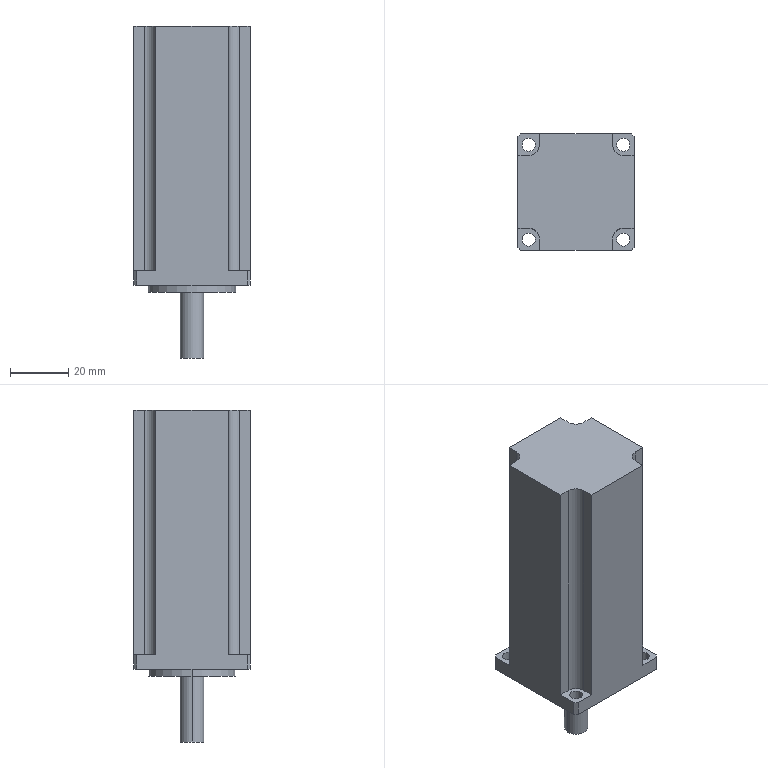Part | Creo | features CURVE 4, DATUM PLANE 3, PROTRUSION 3, CHAMFER 1, COORDINATE SYSTEM 1, CUT 1 | 1 solid | 40 faces | box 40 x 40 x 114 mm | volume 127179 mm3 | plane 24 | cylinder 16 | commonest cylinder face diameters 4.5 x8 7.48 x4 8 x2 30 x2
STEP:
#1=CARTESIAN_POINT('',(0.,0.,0.));
#2=DIRECTION('',(0.,0.,1.));
#3=DIRECTION('',(1.,0.,0.));
#4=AXIS2_PLACEMENT_3D('',#1,#2,#3);
#5=CARTESIAN_POINT('',(19.,20.,0.));
#6=VERTEX_POINT('',#5);
#7=CARTESIAN_POINT('',(20.,19.,0.));
#8=VERTEX_POINT('',#7);
#9=CARTESIAN_POINT('',(19.,20.,0.));
#10=DIRECTION('',(0.7071,-0.7071,0.));
#11=VECTOR('',#10,1.414);
#12=LINE('',#9,#11);
#13=EDGE_CURVE('',#6,#8,#12,.T.);
#14=ORIENTED_EDGE('',*,*,#13,.F.);
#15=CARTESIAN_POINT('',(-19.,20.,0.));
#16=VERTEX_POINT('',#15);
#17=CARTESIAN_POINT('',(19.,20.,0.));
#18=DIRECTION('',(-1.,0.,0.));
#19=VECTOR('',#18,38.);
#20=LINE('',#17,#19);
#21=EDGE_CURVE('',#6,#16,#20,.T.);
#22=ORIENTED_EDGE('',*,*,#21,.T.);
#23=CARTESIAN_POINT('',(-20.,19.,0.));
#24=VERTEX_POINT('',#23);
#25=CARTESIAN_POINT('',(-20.,19.,0.));
#26=DIRECTION('',(0.7071,0.7071,0.));
#27=VECTOR('',#26,1.414);
#28=LINE('',#25,#27);
#29=EDGE_CURVE('',#24,#16,#28,.T.);
#30=ORIENTED_EDGE('',*,*,#29,.F.);
#31=CARTESIAN_POINT('',(-20.,-19.,0.));
#32=VERTEX_POINT('',#31);
#33=CARTESIAN_POINT('',(-20.,19.,0.));
#34=DIRECTION('',(0.,-1.,0.));
#35=VECTOR('',#34,38.);
#36=LINE('',#33,#35);
#37=EDGE_CURVE('',#24,#32,#36,.T.);
#38=ORIENTED_EDGE('',*,*,#37,.T.);
#39=CARTESIAN_POINT('',(-19.,-20.,0.));
#40=VERTEX_POINT('',#39);
#41=CARTESIAN_POINT('',(-19.,-20.,0.));
#42=DIRECTION('',(-0.7071,0.7071,0.));
#43=VECTOR('',#42,1.414);
#44=LINE('',#41,#43);
#45=EDGE_CURVE('',#40,#32,#44,.T.);
#46=ORIENTED_EDGE('',*,*,#45,.F.);
#47=CARTESIAN_POINT('',(19.,-20.,0.));
#48=VERTEX_POINT('',#47);
#49=CARTESIAN_POINT('',(-19.,-20.,0.));
#50=DIRECTION('',(1.,0.,0.));
#51=VECTOR('',#50,38.);
#52=LINE('',#49,#51);
#53=EDGE_CURVE('',#40,#48,#52,.T.);
#54=ORIENTED_EDGE('',*,*,#53,.T.);
#55=CARTESIAN_POINT('',(20.,-19.,0.));
#56=VERTEX_POINT('',#55);
#57=CARTESIAN_POINT('',(20.,-19.,0.));
#58=DIRECTION('',(-0.7071,-0.7071,0.));
#59=VECTOR('',#58,1.414);
#60=LINE('',#57,#59);
#61=EDGE_CURVE('',#56,#48,#60,.T.);
#62=ORIENTED_EDGE('',*,*,#61,.F.);
#63=CARTESIAN_POINT('',(20.,-19.,0.));
#64=DIRECTION('',(0.,1.,0.));
#65=VECTOR('',#64,38.);
#66=LINE('',#63,#65);
#67=EDGE_CURVE('',#56,#8,#66,.T.);
#68=ORIENTED_EDGE('',*,*,#67,.T.);
#69=EDGE_LOOP('',(#14,#22,#30,#38,#46,#54,#62,#68));
#70=FACE_OUTER_BOUND('',#69,.F.);
#71=CARTESIAN_POINT('',(-14.01,16.26,0.));
#72=VERTEX_POINT('',#71);
#73=CARTESIAN_POINT('',(-18.51,16.26,0.));
#74=VERTEX_POINT('',#73);
#75=CARTESIAN_POINT('',(-16.26,16.26,0.));
#76=DIRECTION('',(0.,0.,-1.));
#77=DIRECTION('',(1.,0.,0.));
#78=AXIS2_PLACEMENT_3D('',#75,#76,#77);
#79=CIRCLE('',#78,2.25);
#80=EDGE_CURVE('',#72,#74,#79,.T.);
#81=ORIENTED_EDGE('',*,*,#80,.T.);
#82=CARTESIAN_POINT('',(-16.26,16.26,0.));
#83=DIRECTION('',(0.,0.,-1.));
#84=DIRECTION('',(-1.,0.,0.));
#85=AXIS2_PLACEMENT_3D('',#82,#83,#84);
#86=CIRCLE('',#85,2.25);
#87=EDGE_CURVE('',#74,#72,#86,.T.);
#88=ORIENTED_EDGE('',*,*,#87,.T.);
#89=EDGE_LOOP('',(#81,#88));
#90=FACE_BOUND('',#89,.F.);
#91=CARTESIAN_POINT('',(-14.01,-16.26,0.));
#92=VERTEX_POINT('',#91);
#93=CARTESIAN_POINT('',(-18.51,-16.26,0.));
#94=VERTEX_POINT('',#93);
#95=CARTESIAN_POINT('',(-16.26,-16.26,0.));
#96=DIRECTION('',(0.,0.,-1.));
#97=DIRECTION('',(1.,0.,0.));
#98=AXIS2_PLACEMENT_3D('',#95,#96,#97);
#99=CIRCLE('',#98,2.25);
#100=EDGE_CURVE('',#92,#94,#99,.T.);
#101=ORIENTED_EDGE('',*,*,#100,.T.);
#102=CARTESIAN_POINT('',(-16.26,-16.26,0.));
#103=DIRECTION('',(0.,0.,-1.));
#104=DIRECTION('',(-1.,0.,0.));
#105=AXIS2_PLACEMENT_3D('',#102,#103,#104);
#106=CIRCLE('',#105,2.25);
#107=EDGE_CURVE('',#94,#92,#106,.T.);
#108=ORIENTED_EDGE('',*,*,#107,.T.);
#109=EDGE_LOOP('',(#101,#108));
#110=FACE_BOUND('',#109,.F.);
#111=CARTESIAN_POINT('',(18.51,-16.26,0.));
#112=VERTEX_POINT('',#111);
#113=CARTESIAN_POINT('',(14.01,-16.26,0.));
#114=VERTEX_POINT('',#113);
#115=CARTESIAN_POINT('',(16.26,-16.26,0.));
#116=DIRECTION('',(0.,0.,-1.));
#117=DIRECTION('',(1.,0.,0.));
#118=AXIS2_PLACEMENT_3D('',#115,#116,#117);
#119=CIRCLE('',#118,2.25);
#120=EDGE_CURVE('',#112,#114,#119,.T.);
#121=ORIENTED_EDGE('',*,*,#120,.T.);
#122=CARTESIAN_POINT('',(16.26,-16.26,0.));
#123=DIRECTION('',(0.,0.,-1.));
#124=DIRECTION('',(-1.,0.,0.));
#125=AXIS2_PLACEMENT_3D('',#122,#123,#124);
#126=CIRCLE('',#125,2.25);
#127=EDGE_CURVE('',#114,#112,#126,.T.);
#128=ORIENTED_EDGE('',*,*,#127,.T.);
#129=EDGE_LOOP('',(#121,#128));
#130=FACE_BOUND('',#129,.F.);
#131=CARTESIAN_POINT('',(18.51,16.26,0.));
#132=VERTEX_POINT('',#131);
#133=CARTESIAN_POINT('',(14.01,16.26,0.));
#134=VERTEX_POINT('',#133);
#135=CARTESIAN_POINT('',(16.26,16.26,0.));
#136=DIRECTION('',(0.,0.,-1.));
#137=DIRECTION('',(1.,0.,0.));
#138=AXIS2_PLACEMENT_3D('',#135,#136,#137);
#139=CIRCLE('',#138,2.25);
#140=EDGE_CURVE('',#132,#134,#139,.T.);
#141=ORIENTED_EDGE('',*,*,#140,.T.);
#142=CARTESIAN_POINT('',(16.26,16.26,0.));
#143=DIRECTION('',(0.,0.,-1.));
#144=DIRECTION('',(-1.,0.,0.));
#145=AXIS2_PLACEMENT_3D('',#142,#143,#144);
#146=CIRCLE('',#145,2.25);
#147=EDGE_CURVE('',#134,#132,#146,.T.);
#148=ORIENTED_EDGE('',*,*,#147,.T.);
#149=EDGE_LOOP('',(#141,#148));
#150=FACE_BOUND('',#149,.F.);
#151=CARTESIAN_POINT('',(-15.,0.,0.));
#152=VERTEX_POINT('',#151);
#153=CARTESIAN_POINT('',(15.,0.,0.));
#154=VERTEX_POINT('',#153);
#155=CARTESIAN_POINT('',(0.,0.,0.));
#156=DIRECTION('',(0.,0.,-1.));
#157=DIRECTION('',(-1.,0.,0.));
#158=AXIS2_PLACEMENT_3D('',#155,#156,#157);
#159=CIRCLE('',#158,15.);
#160=EDGE_CURVE('',#152,#154,#159,.T.);
#161=ORIENTED_EDGE('',*,*,#160,.T.);
#162=CARTESIAN_POINT('',(0.,0.,0.));
#163=DIRECTION('',(0.,0.,-1.));
#164=DIRECTION('',(1.,0.,0.));
#165=AXIS2_PLACEMENT_3D('',#162,#163,#164);
#166=CIRCLE('',#165,15.);
#167=EDGE_CURVE('',#154,#152,#166,.T.);
#168=ORIENTED_EDGE('',*,*,#167,.T.);
#169=EDGE_LOOP('',(#161,#168));
#170=FACE_BOUND('',#169,.F.);
#171=CARTESIAN_POINT('',(0.,0.,0.));
#172=DIRECTION('',(0.,0.,1.));
#173=DIRECTION('',(1.,0.,0.));
#174=AXIS2_PLACEMENT_3D('',#171,#172,#173);
#175=PLANE('',#174);
#176=ADVANCED_FACE('',(#70,#90,#110,#130,#150,#170),#175,.F.);
#177=CARTESIAN_POINT('',(14.01,16.26,5.));
#178=VERTEX_POINT('',#177);
#179=CARTESIAN_POINT('',(18.51,16.26,5.));
#180=VERTEX_POINT('',#179);
#181=CARTESIAN_POINT('',(16.26,16.26,5.));
#182=DIRECTION('',(0.,0.,1.));
#183=DIRECTION('',(-1.,0.,0.));
#184=AXIS2_PLACEMENT_3D('',#181,#182,#183);
#185=CIRCLE('',#184,2.25);
#186=EDGE_CURVE('',#178,#180,#185,.T.);
#187=ORIENTED_EDGE('',*,*,#186,.F.);
#188=CARTESIAN_POINT('',(14.01,16.26,0.));
#189=DIRECTION('',(0.,0.,1.));
#190=VECTOR('',#189,5.);
#191=LINE('',#188,#190);
#192=EDGE_CURVE('',#134,#178,#191,.T.);
#193=ORIENTED_EDGE('',*,*,#192,.F.);
#194=ORIENTED_EDGE('',*,*,#140,.F.);
#195=CARTESIAN_POINT('',(18.51,16.26,0.));
#196=DIRECTION('',(0.,0.,1.));
#197=VECTOR('',#196,5.);
#198=LINE('',#195,#197);
#199=EDGE_CURVE('',#132,#180,#198,.T.);
#200=ORIENTED_EDGE('',*,*,#199,.T.);
#201=EDGE_LOOP('',(#187,#193,#194,#200));
#202=FACE_OUTER_BOUND('',#201,.F.);
#203=CARTESIAN_POINT('',(16.26,16.26,0.));
#204=DIRECTION('',(0.,0.,1.));
#205=DIRECTION('',(1.,0.,0.));
#206=AXIS2_PLACEMENT_3D('',#203,#204,#205);
#207=CYLINDRICAL_SURFACE('',#206,2.25);
#208=ADVANCED_FACE('',(#202),#207,.F.);
#209=CARTESIAN_POINT('',(20.,19.,5.));
#210=VERTEX_POINT('',#209);
#211=CARTESIAN_POINT('',(19.,20.,5.));
#212=VERTEX_POINT('',#211);
#213=CARTESIAN_POINT('',(20.,19.,5.));
#214=DIRECTION('',(-0.7071,0.7071,0.));
#215=VECTOR('',#214,1.414);
#216=LINE('',#213,#215);
#217=EDGE_CURVE('',#210,#212,#216,.T.);
#218=ORIENTED_EDGE('',*,*,#217,.F.);
#219=CARTESIAN_POINT('',(20.,12.52,5.));
#220=VERTEX_POINT('',#219);
#221=CARTESIAN_POINT('',(20.,12.52,5.));
#222=DIRECTION('',(0.,1.,0.));
#223=VECTOR('',#222,6.48);
#224=LINE('',#221,#223);
#225=EDGE_CURVE('',#220,#210,#224,.T.);
#226=ORIENTED_EDGE('',*,*,#225,.F.);
#227=CARTESIAN_POINT('',(16.26,12.52,5.));
#228=VERTEX_POINT('',#227);
#229=CARTESIAN_POINT('',(16.26,12.52,5.));
#230=DIRECTION('',(1.,0.,0.));
#231=VECTOR('',#230,3.74);
#232=LINE('',#229,#231);
#233=EDGE_CURVE('',#228,#220,#232,.T.);
#234=ORIENTED_EDGE('',*,*,#233,.F.);
#235=CARTESIAN_POINT('',(12.52,16.26,5.));
#236=VERTEX_POINT('',#235);
#237=CARTESIAN_POINT('',(16.26,16.26,5.));
#238=DIRECTION('',(0.,0.,1.));
#239=DIRECTION('',(-1.,0.,0.));
#240=AXIS2_PLACEMENT_3D('',#237,#238,#239);
#241=CIRCLE('',#240,3.74);
#242=EDGE_CURVE('',#236,#228,#241,.T.);
#243=ORIENTED_EDGE('',*,*,#242,.F.);
#244=CARTESIAN_POINT('',(12.52,20.,5.));
#245=VERTEX_POINT('',#244);
#246=CARTESIAN_POINT('',(12.52,20.,5.));
#247=DIRECTION('',(0.,-1.,0.));
#248=VECTOR('',#247,3.74);
#249=LINE('',#246,#248);
#250=EDGE_CURVE('',#245,#236,#249,.T.);
#251=ORIENTED_EDGE('',*,*,#250,.F.);
#252=CARTESIAN_POINT('',(19.,20.,5.));
#253=DIRECTION('',(-1.,0.,0.));
#254=VECTOR('',#253,6.48);
#255=LINE('',#252,#254);
#256=EDGE_CURVE('',#212,#245,#255,.T.);
#257=ORIENTED_EDGE('',*,*,#256,.F.);
#258=EDGE_LOOP('',(#218,#226,#234,#243,#251,#257));
#259=FACE_OUTER_BOUND('',#258,.F.);
#260=ORIENTED_EDGE('',*,*,#186,.T.);
#261=CARTESIAN_POINT('',(16.26,16.26,5.));
#262=DIRECTION('',(0.,0.,1.));
#263=DIRECTION('',(1.,0.,0.));
#264=AXIS2_PLACEMENT_3D('',#261,#262,#263);
#265=CIRCLE('',#264,2.25);
#266=EDGE_CURVE('',#180,#178,#265,.T.);
#267=ORIENTED_EDGE('',*,*,#266,.T.);
#268=EDGE_LOOP('',(#260,#267));
#269=FACE_BOUND('',#268,.F.);
#270=CARTESIAN_POINT('',(0.,0.,5.));
#271=DIRECTION('',(0.,0.,1.));
#272=DIRECTION('',(1.,0.,0.));
#273=AXIS2_PLACEMENT_3D('',#270,#271,#272);
#274=PLANE('',#273);
#275=ADVANCED_FACE('',(#259,#269),#274,.T.);
#276=CARTESIAN_POINT('',(19.,-20.,5.));
#277=VERTEX_POINT('',#276);
#278=CARTESIAN_POINT('',(20.,-19.,5.));
#279=VERTEX_POINT('',#278);
#280=CARTESIAN_POINT('',(19.,-20.,5.));
#281=DIRECTION('',(0.7071,0.7071,0.));
#282=VECTOR('',#281,1.414);
#283=LINE('',#280,#282);
#284=EDGE_CURVE('',#277,#279,#283,.T.);
#285=ORIENTED_EDGE('',*,*,#284,.F.);
#286=CARTESIAN_POINT('',(12.52,-20.,5.));
#287=VERTEX_POINT('',#286);
#288=CARTESIAN_POINT('',(12.52,-20.,5.));
#289=DIRECTION('',(1.,0.,0.));
#290=VECTOR('',#289,6.48);
#291=LINE('',#288,#290);
#292=EDGE_CURVE('',#287,#277,#291,.T.);
#293=ORIENTED_EDGE('',*,*,#292,.F.);
#294=CARTESIAN_POINT('',(12.52,-16.26,5.));
#295=VERTEX_POINT('',#294);
#296=CARTESIAN_POINT('',(12.52,-16.26,5.));
#297=DIRECTION('',(0.,-1.,0.));
#298=VECTOR('',#297,3.74);
#299=LINE('',#296,#298);
#300=EDGE_CURVE('',#295,#287,#299,.T.);
#301=ORIENTED_EDGE('',*,*,#300,.F.);
#302=CARTESIAN_POINT('',(16.26,-12.52,5.));
#303=VERTEX_POINT('',#302);
#304=CARTESIAN_POINT('',(16.26,-16.26,5.));
#305=DIRECTION('',(0.,0.,1.));
#306=DIRECTION('',(0.,1.,0.));
#307=AXIS2_PLACEMENT_3D('',#304,#305,#306);
#308=CIRCLE('',#307,3.74);
#309=EDGE_CURVE('',#303,#295,#308,.T.);
#310=ORIENTED_EDGE('',*,*,#309,.F.);
#311=CARTESIAN_POINT('',(20.,-12.52,5.));
#312=VERTEX_POINT('',#311);
#313=CARTESIAN_POINT('',(20.,-12.52,5.));
#314=DIRECTION('',(-1.,0.,0.));
#315=VECTOR('',#314,3.74);
#316=LINE('',#313,#315);
#317=EDGE_CURVE('',#312,#303,#316,.T.);
#318=ORIENTED_EDGE('',*,*,#317,.F.);
#319=CARTESIAN_POINT('',(20.,-19.,5.));
#320=DIRECTION('',(0.,1.,0.));
#321=VECTOR('',#320,6.48);
#322=LINE('',#319,#321);
#323=EDGE_CURVE('',#279,#312,#322,.T.);
#324=ORIENTED_EDGE('',*,*,#323,.F.);
#325=EDGE_LOOP('',(#285,#293,#301,#310,#318,#324));
#326=FACE_OUTER_BOUND('',#325,.F.);
#327=CARTESIAN_POINT('',(14.01,-16.26,5.));
#328=VERTEX_POINT('',#327);
#329=CARTESIAN_POINT('',(18.51,-16.26,5.));
#330=VERTEX_POINT('',#329);
#331=CARTESIAN_POINT('',(16.26,-16.26,5.));
#332=DIRECTION('',(0.,0.,1.));
#333=DIRECTION('',(-1.,0.,0.));
#334=AXIS2_PLACEMENT_3D('',#331,#332,#333);
#335=CIRCLE('',#334,2.25);
#336=EDGE_CURVE('',#328,#330,#335,.T.);
#337=ORIENTED_EDGE('',*,*,#336,.T.);
#338=CARTESIAN_POINT('',(16.26,-16.26,5.));
#339=DIRECTION('',(0.,0.,1.));
#340=DIRECTION('',(1.,0.,0.));
#341=AXIS2_PLACEMENT_3D('',#338,#339,#340);
#342=CIRCLE('',#341,2.25);
#343=EDGE_CURVE('',#330,#328,#342,.T.);
#344=ORIENTED_EDGE('',*,*,#343,.T.);
#345=EDGE_LOOP('',(#337,#344));
#346=FACE_BOUND('',#345,.F.);
#347=CARTESIAN_POINT('',(0.,0.,5.));
#348=DIRECTION('',(0.,0.,1.));
#349=DIRECTION('',(1.,0.,0.));
#350=AXIS2_PLACEMENT_3D('',#347,#348,#349);
#351=PLANE('',#350);
#352=ADVANCED_FACE('',(#326,#346),#351,.T.);
#353=CARTESIAN_POINT('',(-20.,-19.,5.));
#354=VERTEX_POINT('',#353);
#355=CARTESIAN_POINT('',(-19.,-20.,5.));
#356=VERTEX_POINT('',#355);
#357=CARTESIAN_POINT('',(-20.,-19.,5.));
#358=DIRECTION('',(0.7071,-0.7071,0.));
#359=VECTOR('',#358,1.414);
#360=LINE('',#357,#359);
#361=EDGE_CURVE('',#354,#356,#360,.T.);
#362=ORIENTED_EDGE('',*,*,#361,.F.);
#363=CARTESIAN_POINT('',(-20.,-12.52,5.));
#364=VERTEX_POINT('',#363);
#365=CARTESIAN_POINT('',(-20.,-12.52,5.));
#366=DIRECTION('',(0.,-1.,0.));
#367=VECTOR('',#366,6.48);
#368=LINE('',#365,#367);
#369=EDGE_CURVE('',#364,#354,#368,.T.);
#370=ORIENTED_EDGE('',*,*,#369,.F.);
#371=CARTESIAN_POINT('',(-16.26,-12.52,5.));
#372=VERTEX_POINT('',#371);
#373=CARTESIAN_POINT('',(-16.26,-12.52,5.));
#374=DIRECTION('',(-1.,0.,0.));
#375=VECTOR('',#374,3.74);
#376=LINE('',#373,#375);
#377=EDGE_CURVE('',#372,#364,#376,.T.);
#378=ORIENTED_EDGE('',*,*,#377,.F.);
#379=CARTESIAN_POINT('',(-12.52,-16.26,5.));
#380=VERTEX_POINT('',#379);
#381=CARTESIAN_POINT('',(-16.26,-16.26,5.));
#382=DIRECTION('',(0.,0.,1.));
#383=DIRECTION('',(1.,0.,0.));
#384=AXIS2_PLACEMENT_3D('',#381,#382,#383);
#385=CIRCLE('',#384,3.74);
#386=EDGE_CURVE('',#380,#372,#385,.T.);
#387=ORIENTED_EDGE('',*,*,#386,.F.);
#388=CARTESIAN_POINT('',(-12.52,-20.,5.));
#389=VERTEX_POINT('',#388);
#390=CARTESIAN_POINT('',(-12.52,-20.,5.));
#391=DIRECTION('',(0.,1.,0.));
#392=VECTOR('',#391,3.74);
#393=LINE('',#390,#392);
#394=EDGE_CURVE('',#389,#380,#393,.T.);
#395=ORIENTED_EDGE('',*,*,#394,.F.);
#396=CARTESIAN_POINT('',(-19.,-20.,5.));
#397=DIRECTION('',(1.,0.,0.));
#398=VECTOR('',#397,6.48);
#399=LINE('',#396,#398);
#400=EDGE_CURVE('',#356,#389,#399,.T.);
#401=ORIENTED_EDGE('',*,*,#400,.F.);
#402=EDGE_LOOP('',(#362,#370,#378,#387,#395,#401));
#403=FACE_OUTER_BOUND('',#402,.F.);
#404=CARTESIAN_POINT('',(-18.51,-16.26,5.));
#405=VERTEX_POINT('',#404);
#406=CARTESIAN_POINT('',(-14.01,-16.26,5.));
#407=VERTEX_POINT('',#406);
#408=CARTESIAN_POINT('',(-16.26,-16.26,5.));
#409=DIRECTION('',(0.,0.,1.));
#410=DIRECTION('',(-1.,0.,0.));
#411=AXIS2_PLACEMENT_3D('',#408,#409,#410);
#412=CIRCLE('',#411,2.25);
#413=EDGE_CURVE('',#405,#407,#412,.T.);
#414=ORIENTED_EDGE('',*,*,#413,.T.);
#415=CARTESIAN_POINT('',(-16.26,-16.26,5.));
#416=DIRECTION('',(0.,0.,1.));
#417=DIRECTION('',(1.,0.,0.));
#418=AXIS2_PLACEMENT_3D('',#415,#416,#417);
#419=CIRCLE('',#418,2.25);
#420=EDGE_CURVE('',#407,#405,#419,.T.);
#421=ORIENTED_EDGE('',*,*,#420,.T.);
#422=EDGE_LOOP('',(#414,#421));
#423=FACE_BOUND('',#422,.F.);
#424=CARTESIAN_POINT('',(0.,0.,5.));
#425=DIRECTION('',(0.,0.,1.));
#426=DIRECTION('',(1.,0.,0.));
#427=AXIS2_PLACEMENT_3D('',#424,#425,#426);
#428=PLANE('',#427);
#429=ADVANCED_FACE('',(#403,#423),#428,.T.);
#430=CARTESIAN_POINT('',(-19.,20.,5.));
#431=VERTEX_POINT('',#430);
#432=CARTESIAN_POINT('',(-20.,19.,5.));
#433=VERTEX_POINT('',#432);
#434=CARTESIAN_POINT('',(-19.,20.,5.));
#435=DIRECTION('',(-0.7071,-0.7071,0.));
#436=VECTOR('',#435,1.414);
#437=LINE('',#434,#436);
#438=EDGE_CURVE('',#431,#433,#437,.T.);
#439=ORIENTED_EDGE('',*,*,#438,.F.);
#440=CARTESIAN_POINT('',(-12.52,20.,5.));
#441=VERTEX_POINT('',#440);
#442=CARTESIAN_POINT('',(-12.52,20.,5.));
#443=DIRECTION('',(-1.,0.,0.));
#444=VECTOR('',#443,6.48);
#445=LINE('',#442,#444);
#446=EDGE_CURVE('',#441,#431,#445,.T.);
#447=ORIENTED_EDGE('',*,*,#446,.F.);
#448=CARTESIAN_POINT('',(-12.52,16.26,5.));
#449=VERTEX_POINT('',#448);
#450=CARTESIAN_POINT('',(-12.52,16.26,5.));
#451=DIRECTION('',(0.,1.,0.));
#452=VECTOR('',#451,3.74);
#453=LINE('',#450,#452);
#454=EDGE_CURVE('',#449,#441,#453,.T.);
#455=ORIENTED_EDGE('',*,*,#454,.F.);
#456=CARTESIAN_POINT('',(-16.26,12.52,5.));
#457=VERTEX_POINT('',#456);
#458=CARTESIAN_POINT('',(-16.26,16.26,5.));
#459=DIRECTION('',(0.,0.,1.));
#460=DIRECTION('',(0.,-1.,0.));
#461=AXIS2_PLACEMENT_3D('',#458,#459,#460);
#462=CIRCLE('',#461,3.74);
#463=EDGE_CURVE('',#457,#449,#462,.T.);
#464=ORIENTED_EDGE('',*,*,#463,.F.);
#465=CARTESIAN_POINT('',(-20.,12.52,5.));
#466=VERTEX_POINT('',#465);
#467=CARTESIAN_POINT('',(-20.,12.52,5.));
#468=DIRECTION('',(1.,0.,0.));
#469=VECTOR('',#468,3.74);
#470=LINE('',#467,#469);
#471=EDGE_CURVE('',#466,#457,#470,.T.);
#472=ORIENTED_EDGE('',*,*,#471,.F.);
#473=CARTESIAN_POINT('',(-20.,19.,5.));
#474=DIRECTION('',(0.,-1.,0.));
#475=VECTOR('',#474,6.48);
#476=LINE('',#473,#475);
#477=EDGE_CURVE('',#433,#466,#476,.T.);
#478=ORIENTED_EDGE('',*,*,#477,.F.);
#479=EDGE_LOOP('',(#439,#447,#455,#464,#472,#478));
#480=FACE_OUTER_BOUND('',#479,.F.);
#481=CARTESIAN_POINT('',(-18.51,16.26,5.));
#482=VERTEX_POINT('',#481);
#483=CARTESIAN_POINT('',(-14.01,16.26,5.));
#484=VERTEX_POINT('',#483);
#485=CARTESIAN_POINT('',(-16.26,16.26,5.));
#486=DIRECTION('',(0.,0.,1.));
#487=DIRECTION('',(-1.,0.,0.));
#488=AXIS2_PLACEMENT_3D('',#485,#486,#487);
#489=CIRCLE('',#488,2.25);
#490=EDGE_CURVE('',#482,#484,#489,.T.);
#491=ORIENTED_EDGE('',*,*,#490,.T.);
#492=CARTESIAN_POINT('',(-16.26,16.26,5.));
#493=DIRECTION('',(0.,0.,1.));
#494=DIRECTION('',(1.,0.,0.));
#495=AXIS2_PLACEMENT_3D('',#492,#493,#494);
#496=CIRCLE('',#495,2.25);
#497=EDGE_CURVE('',#484,#482,#496,.T.);
#498=ORIENTED_EDGE('',*,*,#497,.T.);
#499=EDGE_LOOP('',(#491,#498));
#500=FACE_BOUND('',#499,.F.);
#501=CARTESIAN_POINT('',(0.,0.,5.));
#502=DIRECTION('',(0.,0.,1.));
#503=DIRECTION('',(1.,0.,0.));
#504=AXIS2_PLACEMENT_3D('',#501,#502,#503);
#505=PLANE('',#504);
#506=ADVANCED_FACE('',(#480,#500),#505,.T.);
#507=ORIENTED_EDGE('',*,*,#336,.F.);
#508=CARTESIAN_POINT('',(14.01,-16.26,0.));
#509=DIRECTION('',(0.,0.,1.));
#510=VECTOR('',#509,5.);
#511=LINE('',#508,#510);
#512=EDGE_CURVE('',#114,#328,#511,.T.);
#513=ORIENTED_EDGE('',*,*,#512,.F.);
#514=ORIENTED_EDGE('',*,*,#120,.F.);
#515=CARTESIAN_POINT('',(18.51,-16.26,0.));
#516=DIRECTION('',(0.,0.,1.));
#517=VECTOR('',#516,5.);
#518=LINE('',#515,#517);
#519=EDGE_CURVE('',#112,#330,#518,.T.);
#520=ORIENTED_EDGE('',*,*,#519,.T.);
#521=EDGE_LOOP('',(#507,#513,#514,#520));
#522=FACE_OUTER_BOUND('',#521,.F.);
#523=CARTESIAN_POINT('',(16.26,-16.26,0.));
#524=DIRECTION('',(0.,0.,1.));
#525=DIRECTION('',(1.,0.,0.));
#526=AXIS2_PLACEMENT_3D('',#523,#524,#525);
#527=CYLINDRICAL_SURFACE('',#526,2.25);
#528=ADVANCED_FACE('',(#522),#527,.F.);
#529=ORIENTED_EDGE('',*,*,#343,.F.);
#530=ORIENTED_EDGE('',*,*,#519,.F.);
#531=ORIENTED_EDGE('',*,*,#127,.F.);
#532=ORIENTED_EDGE('',*,*,#512,.T.);
#533=EDGE_LOOP('',(#529,#530,#531,#532));
#534=FACE_OUTER_BOUND('',#533,.F.);
#535=CARTESIAN_POINT('',(16.26,-16.26,0.));
#536=DIRECTION('',(0.,0.,1.));
#537=DIRECTION('',(1.,0.,0.));
#538=AXIS2_PLACEMENT_3D('',#535,#536,#537);
#539=CYLINDRICAL_SURFACE('',#538,2.25);
#540=ADVANCED_FACE('',(#534),#539,.F.);
#541=ORIENTED_EDGE('',*,*,#266,.F.);
#542=ORIENTED_EDGE('',*,*,#199,.F.);
#543=ORIENTED_EDGE('',*,*,#147,.F.);
#544=ORIENTED_EDGE('',*,*,#192,.T.);
#545=EDGE_LOOP('',(#541,#542,#543,#544));
#546=FACE_OUTER_BOUND('',#545,.F.);
#547=CARTESIAN_POINT('',(16.26,16.26,0.));
#548=DIRECTION('',(0.,0.,1.));
#549=DIRECTION('',(1.,0.,0.));
#550=AXIS2_PLACEMENT_3D('',#547,#548,#549);
#551=CYLINDRICAL_SURFACE('',#550,2.25);
#552=ADVANCED_FACE('',(#546),#551,.F.);
#553=ORIENTED_EDGE('',*,*,#490,.F.);
#554=CARTESIAN_POINT('',(-18.51,16.26,0.));
#555=DIRECTION('',(0.,0.,1.));
#556=VECTOR('',#555,5.);
#557=LINE('',#554,#556);
#558=EDGE_CURVE('',#74,#482,#557,.T.);
#559=ORIENTED_EDGE('',*,*,#558,.F.);
#560=ORIENTED_EDGE('',*,*,#80,.F.);
#561=CARTESIAN_POINT('',(-14.01,16.26,0.));
#562=DIRECTION('',(0.,0.,1.));
#563=VECTOR('',#562,5.);
#564=LINE('',#561,#563);
#565=EDGE_CURVE('',#72,#484,#564,.T.);
#566=ORIENTED_EDGE('',*,*,#565,.T.);
#567=EDGE_LOOP('',(#553,#559,#560,#566));
#568=FACE_OUTER_BOUND('',#567,.F.);
#569=CARTESIAN_POINT('',(-16.26,16.26,0.));
#570=DIRECTION('',(0.,0.,1.));
#571=DIRECTION('',(1.,0.,0.));
#572=AXIS2_PLACEMENT_3D('',#569,#570,#571);
#573=CYLINDRICAL_SURFACE('',#572,2.25);
#574=ADVANCED_FACE('',(#568),#573,.F.);
#575=ORIENTED_EDGE('',*,*,#497,.F.);
#576=ORIENTED_EDGE('',*,*,#565,.F.);
#577=ORIENTED_EDGE('',*,*,#87,.F.);
#578=ORIENTED_EDGE('',*,*,#558,.T.);
#579=EDGE_LOOP('',(#575,#576,#577,#578));
#580=FACE_OUTER_BOUND('',#579,.F.);
#581=CARTESIAN_POINT('',(-16.26,16.26,0.));
#582=DIRECTION('',(0.,0.,1.));
#583=DIRECTION('',(1.,0.,0.));
#584=AXIS2_PLACEMENT_3D('',#581,#582,#583);
#585=CYLINDRICAL_SURFACE('',#584,2.25);
#586=ADVANCED_FACE('',(#580),#585,.F.);
#587=ORIENTED_EDGE('',*,*,#413,.F.);
#588=CARTESIAN_POINT('',(-18.51,-16.26,0.));
#589=DIRECTION('',(0.,0.,1.));
#590=VECTOR('',#589,5.);
#591=LINE('',#588,#590);
#592=EDGE_CURVE('',#94,#405,#591,.T.);
#593=ORIENTED_EDGE('',*,*,#592,.F.);
#594=ORIENTED_EDGE('',*,*,#100,.F.);
#595=CARTESIAN_POINT('',(-14.01,-16.26,0.));
#596=DIRECTION('',(0.,0.,1.));
#597=VECTOR('',#596,5.);
#598=LINE('',#595,#597);
#599=EDGE_CURVE('',#92,#407,#598,.T.);
#600=ORIENTED_EDGE('',*,*,#599,.T.);
#601=EDGE_LOOP('',(#587,#593,#594,#600));
#602=FACE_OUTER_BOUND('',#601,.F.);
#603=CARTESIAN_POINT('',(-16.26,-16.26,0.));
#604=DIRECTION('',(0.,0.,1.));
#605=DIRECTION('',(1.,0.,0.));
#606=AXIS2_PLACEMENT_3D('',#603,#604,#605);
#607=CYLINDRICAL_SURFACE('',#606,2.25);
#608=ADVANCED_FACE('',(#602),#607,.F.);
#609=ORIENTED_EDGE('',*,*,#420,.F.);
#610=ORIENTED_EDGE('',*,*,#599,.F.);
#611=ORIENTED_EDGE('',*,*,#107,.F.);
#612=ORIENTED_EDGE('',*,*,#592,.T.);
#613=EDGE_LOOP('',(#609,#610,#611,#612));
#614=FACE_OUTER_BOUND('',#613,.F.);
#615=CARTESIAN_POINT('',(-16.26,-16.26,0.));
#616=DIRECTION('',(0.,0.,1.));
#617=DIRECTION('',(1.,0.,0.));
#618=AXIS2_PLACEMENT_3D('',#615,#616,#617);
#619=CYLINDRICAL_SURFACE('',#618,2.25);
#620=ADVANCED_FACE('',(#614),#619,.F.);
#621=ORIENTED_EDGE('',*,*,#13,.T.);
#622=CARTESIAN_POINT('',(20.,19.,5.));
#623=DIRECTION('',(0.,0.,-1.));
#624=VECTOR('',#623,5.);
#625=LINE('',#622,#624);
#626=EDGE_CURVE('',#210,#8,#625,.T.);
#627=ORIENTED_EDGE('',*,*,#626,.F.);
#628=ORIENTED_EDGE('',*,*,#217,.T.);
#629=CARTESIAN_POINT('',(19.,20.,5.));
#630=DIRECTION('',(0.,0.,-1.));
#631=VECTOR('',#630,5.);
#632=LINE('',#629,#631);
#633=EDGE_CURVE('',#212,#6,#632,.T.);
#634=ORIENTED_EDGE('',*,*,#633,.T.);
#635=EDGE_LOOP('',(#621,#627,#628,#634));
#636=FACE_OUTER_BOUND('',#635,.F.);
#637=CARTESIAN_POINT('',(19.5,19.5,2.5));
#638=DIRECTION('',(0.7071,0.7071,0.));
#639=DIRECTION('',(0.7071,-0.7071,0.));
#640=AXIS2_PLACEMENT_3D('',#637,#638,#639);
#641=PLANE('',#640);
#642=ADVANCED_FACE('',(#636),#641,.T.);
#643=ORIENTED_EDGE('',*,*,#626,.T.);
#644=ORIENTED_EDGE('',*,*,#67,.F.);
#645=CARTESIAN_POINT('',(20.,-19.,5.));
#646=DIRECTION('',(0.,0.,-1.));
#647=VECTOR('',#646,5.);
#648=LINE('',#645,#647);
#649=EDGE_CURVE('',#279,#56,#648,.T.);
#650=ORIENTED_EDGE('',*,*,#649,.F.);
#651=ORIENTED_EDGE('',*,*,#323,.T.);
#652=CARTESIAN_POINT('',(20.,-12.52,89.));
#653=VERTEX_POINT('',#652);
#654=CARTESIAN_POINT('',(20.,-12.52,89.));
#655=DIRECTION('',(0.,0.,-1.));
#656=VECTOR('',#655,84.);
#657=LINE('',#654,#656);
#658=EDGE_CURVE('',#653,#312,#657,.T.);
#659=ORIENTED_EDGE('',*,*,#658,.F.);
#660=CARTESIAN_POINT('',(20.,12.52,89.));
#661=VERTEX_POINT('',#660);
#662=CARTESIAN_POINT('',(20.,-12.52,89.));
#663=DIRECTION('',(0.,1.,0.));
#664=VECTOR('',#663,25.04);
#665=LINE('',#662,#664);
#666=EDGE_CURVE('',#653,#661,#665,.T.);
#667=ORIENTED_EDGE('',*,*,#666,.T.);
#668=CARTESIAN_POINT('',(20.,12.52,89.));
#669=DIRECTION('',(0.,0.,-1.));
#670=VECTOR('',#669,84.);
#671=LINE('',#668,#670);
#672=EDGE_CURVE('',#661,#220,#671,.T.);
#673=ORIENTED_EDGE('',*,*,#672,.T.);
#674=ORIENTED_EDGE('',*,*,#225,.T.);
#675=EDGE_LOOP('',(#643,#644,#650,#651,#659,#667,#673,#674));
#676=FACE_OUTER_BOUND('',#675,.F.);
#677=CARTESIAN_POINT('',(20.,-20.,0.));
#678=DIRECTION('',(1.,0.,0.));
#679=DIRECTION('',(0.,1.,0.));
#680=AXIS2_PLACEMENT_3D('',#677,#678,#679);
#681=PLANE('',#680);
#682=ADVANCED_FACE('',(#676),#681,.T.);
#683=ORIENTED_EDGE('',*,*,#61,.T.);
#684=CARTESIAN_POINT('',(19.,-20.,5.));
#685=DIRECTION('',(0.,0.,-1.));
#686=VECTOR('',#685,5.);
#687=LINE('',#684,#686);
#688=EDGE_CURVE('',#277,#48,#687,.T.);
#689=ORIENTED_EDGE('',*,*,#688,.F.);
#690=ORIENTED_EDGE('',*,*,#284,.T.);
#691=ORIENTED_EDGE('',*,*,#649,.T.);
#692=EDGE_LOOP('',(#683,#689,#690,#691));
#693=FACE_OUTER_BOUND('',#692,.F.);
#694=CARTESIAN_POINT('',(19.5,-19.5,2.5));
#695=DIRECTION('',(0.7071,-0.7071,0.));
#696=DIRECTION('',(-0.7071,-0.7071,0.));
#697=AXIS2_PLACEMENT_3D('',#694,#695,#696);
#698=PLANE('',#697);
#699=ADVANCED_FACE('',(#693),#698,.T.);
#700=ORIENTED_EDGE('',*,*,#688,.T.);
#701=ORIENTED_EDGE('',*,*,#53,.F.);
#702=CARTESIAN_POINT('',(-19.,-20.,5.));
#703=DIRECTION('',(0.,0.,-1.));
#704=VECTOR('',#703,5.);
#705=LINE('',#702,#704);
#706=EDGE_CURVE('',#356,#40,#705,.T.);
#707=ORIENTED_EDGE('',*,*,#706,.F.);
#708=ORIENTED_EDGE('',*,*,#400,.T.);
#709=CARTESIAN_POINT('',(-12.52,-20.,89.));
#710=VERTEX_POINT('',#709);
#711=CARTESIAN_POINT('',(-12.52,-20.,89.));
#712=DIRECTION('',(0.,0.,-1.));
#713=VECTOR('',#712,84.);
#714=LINE('',#711,#713);
#715=EDGE_CURVE('',#710,#389,#714,.T.);
#716=ORIENTED_EDGE('',*,*,#715,.F.);
#717=CARTESIAN_POINT('',(12.52,-20.,89.));
#718=VERTEX_POINT('',#717);
#719=CARTESIAN_POINT('',(-12.52,-20.,89.));
#720=DIRECTION('',(1.,0.,0.));
#721=VECTOR('',#720,25.04);
#722=LINE('',#719,#721);
#723=EDGE_CURVE('',#710,#718,#722,.T.);
#724=ORIENTED_EDGE('',*,*,#723,.T.);
#725=CARTESIAN_POINT('',(12.52,-20.,89.));
#726=DIRECTION('',(0.,0.,-1.));
#727=VECTOR('',#726,84.);
#728=LINE('',#725,#727);
#729=EDGE_CURVE('',#718,#287,#728,.T.);
#730=ORIENTED_EDGE('',*,*,#729,.T.);
#731=ORIENTED_EDGE('',*,*,#292,.T.);
#732=EDGE_LOOP('',(#700,#701,#707,#708,#716,#724,#730,#731));
#733=FACE_OUTER_BOUND('',#732,.F.);
#734=CARTESIAN_POINT('',(-20.,-20.,0.));
#735=DIRECTION('',(0.,-1.,0.));
#736=DIRECTION('',(1.,0.,0.));
#737=AXIS2_PLACEMENT_3D('',#734,#735,#736);
#738=PLANE('',#737);
#739=ADVANCED_FACE('',(#733),#738,.T.);
#740=ORIENTED_EDGE('',*,*,#45,.T.);
#741=CARTESIAN_POINT('',(-20.,-19.,5.));
#742=DIRECTION('',(0.,0.,-1.));
#743=VECTOR('',#742,5.);
#744=LINE('',#741,#743);
#745=EDGE_CURVE('',#354,#32,#744,.T.);
#746=ORIENTED_EDGE('',*,*,#745,.F.);
#747=ORIENTED_EDGE('',*,*,#361,.T.);
#748=ORIENTED_EDGE('',*,*,#706,.T.);
#749=EDGE_LOOP('',(#740,#746,#747,#748));
#750=FACE_OUTER_BOUND('',#749,.F.);
#751=CARTESIAN_POINT('',(-19.5,-19.5,2.5));
#752=DIRECTION('',(-0.7071,-0.7071,0.));
#753=DIRECTION('',(-0.7071,0.7071,0.));
#754=AXIS2_PLACEMENT_3D('',#751,#752,#753);
#755=PLANE('',#754);
#756=ADVANCED_FACE('',(#750),#755,.T.);
#757=ORIENTED_EDGE('',*,*,#745,.T.);
#758=ORIENTED_EDGE('',*,*,#37,.F.);
#759=CARTESIAN_POINT('',(-20.,19.,5.));
#760=DIRECTION('',(0.,0.,-1.));
#761=VECTOR('',#760,5.);
#762=LINE('',#759,#761);
#763=EDGE_CURVE('',#433,#24,#762,.T.);
#764=ORIENTED_EDGE('',*,*,#763,.F.);
#765=ORIENTED_EDGE('',*,*,#477,.T.);
#766=CARTESIAN_POINT('',(-20.,12.52,89.));
#767=VERTEX_POINT('',#766);
#768=CARTESIAN_POINT('',(-20.,12.52,89.));
#769=DIRECTION('',(0.,0.,-1.));
#770=VECTOR('',#769,84.);
#771=LINE('',#768,#770);
#772=EDGE_CURVE('',#767,#466,#771,.T.);
#773=ORIENTED_EDGE('',*,*,#772,.F.);
#774=CARTESIAN_POINT('',(-20.,-12.52,89.));
#775=VERTEX_POINT('',#774);
#776=CARTESIAN_POINT('',(-20.,12.52,89.));
#777=DIRECTION('',(0.,-1.,0.));
#778=VECTOR('',#777,25.04);
#779=LINE('',#776,#778);
#780=EDGE_CURVE('',#767,#775,#779,.T.);
#781=ORIENTED_EDGE('',*,*,#780,.T.);
#782=CARTESIAN_POINT('',(-20.,-12.52,89.));
#783=DIRECTION('',(0.,0.,-1.));
#784=VECTOR('',#783,84.);
#785=LINE('',#782,#784);
#786=EDGE_CURVE('',#775,#364,#785,.T.);
#787=ORIENTED_EDGE('',*,*,#786,.T.);
#788=ORIENTED_EDGE('',*,*,#369,.T.);
#789=EDGE_LOOP('',(#757,#758,#764,#765,#773,#781,#787,#788));
#790=FACE_OUTER_BOUND('',#789,.F.);
#791=CARTESIAN_POINT('',(-20.,20.,0.));
#792=DIRECTION('',(-1.,0.,0.));
#793=DIRECTION('',(0.,-1.,0.));
#794=AXIS2_PLACEMENT_3D('',#791,#792,#793);
#795=PLANE('',#794);
#796=ADVANCED_FACE('',(#790),#795,.T.);
#797=ORIENTED_EDGE('',*,*,#29,.T.);
#798=CARTESIAN_POINT('',(-19.,20.,5.));
#799=DIRECTION('',(0.,0.,-1.));
#800=VECTOR('',#799,5.);
#801=LINE('',#798,#800);
#802=EDGE_CURVE('',#431,#16,#801,.T.);
#803=ORIENTED_EDGE('',*,*,#802,.F.);
#804=ORIENTED_EDGE('',*,*,#438,.T.);
#805=ORIENTED_EDGE('',*,*,#763,.T.);
#806=EDGE_LOOP('',(#797,#803,#804,#805));
#807=FACE_OUTER_BOUND('',#806,.F.);
#808=CARTESIAN_POINT('',(-19.5,19.5,2.5));
#809=DIRECTION('',(-0.7071,0.7071,0.));
#810=DIRECTION('',(0.7071,0.7071,0.));
#811=AXIS2_PLACEMENT_3D('',#808,#809,#810);
#812=PLANE('',#811);
#813=ADVANCED_FACE('',(#807),#812,.T.);
#814=ORIENTED_EDGE('',*,*,#633,.F.);
#815=ORIENTED_EDGE('',*,*,#256,.T.);
#816=CARTESIAN_POINT('',(12.52,20.,89.));
#817=VERTEX_POINT('',#816);
#818=CARTESIAN_POINT('',(12.52,20.,89.));
#819=DIRECTION('',(0.,0.,-1.));
#820=VECTOR('',#819,84.);
#821=LINE('',#818,#820);
#822=EDGE_CURVE('',#817,#245,#821,.T.);
#823=ORIENTED_EDGE('',*,*,#822,.F.);
#824=CARTESIAN_POINT('',(-12.52,20.,89.));
#825=VERTEX_POINT('',#824);
#826=CARTESIAN_POINT('',(12.52,20.,89.));
#827=DIRECTION('',(-1.,0.,0.));
#828=VECTOR('',#827,25.04);
#829=LINE('',#826,#828);
#830=EDGE_CURVE('',#817,#825,#829,.T.);
#831=ORIENTED_EDGE('',*,*,#830,.T.);
#832=CARTESIAN_POINT('',(-12.52,20.,89.));
#833=DIRECTION('',(0.,0.,-1.));
#834=VECTOR('',#833,84.);
#835=LINE('',#832,#834);
#836=EDGE_CURVE('',#825,#441,#835,.T.);
#837=ORIENTED_EDGE('',*,*,#836,.T.);
#838=ORIENTED_EDGE('',*,*,#446,.T.);
#839=ORIENTED_EDGE('',*,*,#802,.T.);
#840=ORIENTED_EDGE('',*,*,#21,.F.);
#841=EDGE_LOOP('',(#814,#815,#823,#831,#837,#838,#839,#840));
#842=FACE_OUTER_BOUND('',#841,.F.);
#843=CARTESIAN_POINT('',(20.,20.,0.));
#844=DIRECTION('',(0.,1.,0.));
#845=DIRECTION('',(-1.,0.,0.));
#846=AXIS2_PLACEMENT_3D('',#843,#844,#845);
#847=PLANE('',#846);
#848=ADVANCED_FACE('',(#842),#847,.T.);
#849=CARTESIAN_POINT('',(12.52,16.26,89.));
#850=VERTEX_POINT('',#849);
#851=CARTESIAN_POINT('',(12.52,20.,89.));
#852=DIRECTION('',(0.,-1.,0.));
#853=VECTOR('',#852,3.74);
#854=LINE('',#851,#853);
#855=EDGE_CURVE('',#817,#850,#854,.T.);
#856=ORIENTED_EDGE('',*,*,#855,.F.);
#857=ORIENTED_EDGE('',*,*,#822,.T.);
#858=ORIENTED_EDGE('',*,*,#250,.T.);
#859=CARTESIAN_POINT('',(12.52,16.26,89.));
#860=DIRECTION('',(0.,0.,-1.));
#861=VECTOR('',#860,84.);
#862=LINE('',#859,#861);
#863=EDGE_CURVE('',#850,#236,#862,.T.);
#864=ORIENTED_EDGE('',*,*,#863,.F.);
#865=EDGE_LOOP('',(#856,#857,#858,#864));
#866=FACE_OUTER_BOUND('',#865,.F.);
#867=CARTESIAN_POINT('',(12.52,20.,89.));
#868=DIRECTION('',(-1.,0.,0.));
#869=DIRECTION('',(0.,-1.,0.));
#870=AXIS2_PLACEMENT_3D('',#867,#868,#869);
#871=PLANE('',#870);
#872=ADVANCED_FACE('',(#866),#871,.F.);
#873=ORIENTED_EDGE('',*,*,#855,.T.);
#874=CARTESIAN_POINT('',(16.26,12.52,89.));
#875=VERTEX_POINT('',#874);
#876=CARTESIAN_POINT('',(16.26,16.26,89.));
#877=DIRECTION('',(0.,0.,1.));
#878=DIRECTION('',(-1.,0.,0.));
#879=AXIS2_PLACEMENT_3D('',#876,#877,#878);
#880=CIRCLE('',#879,3.74);
#881=EDGE_CURVE('',#850,#875,#880,.T.);
#882=ORIENTED_EDGE('',*,*,#881,.T.);
#883=CARTESIAN_POINT('',(20.,12.52,89.));
#884=DIRECTION('',(-1.,0.,0.));
#885=VECTOR('',#884,3.74);
#886=LINE('',#883,#885);
#887=EDGE_CURVE('',#661,#875,#886,.T.);
#888=ORIENTED_EDGE('',*,*,#887,.F.);
#889=ORIENTED_EDGE('',*,*,#666,.F.);
#890=CARTESIAN_POINT('',(16.26,-12.52,89.));
#891=VERTEX_POINT('',#890);
#892=CARTESIAN_POINT('',(20.,-12.52,89.));
#893=DIRECTION('',(-1.,0.,0.));
#894=VECTOR('',#893,3.74);
#895=LINE('',#892,#894);
#896=EDGE_CURVE('',#653,#891,#895,.T.);
#897=ORIENTED_EDGE('',*,*,#896,.T.);
#898=CARTESIAN_POINT('',(12.52,-16.26,89.));
#899=VERTEX_POINT('',#898);
#900=CARTESIAN_POINT('',(16.26,-16.26,89.));
#901=DIRECTION('',(0.,0.,1.));
#902=DIRECTION('',(0.,1.,0.));
#903=AXIS2_PLACEMENT_3D('',#900,#901,#902);
#904=CIRCLE('',#903,3.74);
#905=EDGE_CURVE('',#891,#899,#904,.T.);
#906=ORIENTED_EDGE('',*,*,#905,.T.);
#907=CARTESIAN_POINT('',(12.52,-20.,89.));
#908=DIRECTION('',(0.,1.,0.));
#909=VECTOR('',#908,3.74);
#910=LINE('',#907,#909);
#911=EDGE_CURVE('',#718,#899,#910,.T.);
#912=ORIENTED_EDGE('',*,*,#911,.F.);
#913=ORIENTED_EDGE('',*,*,#723,.F.);
#914=CARTESIAN_POINT('',(-12.52,-16.26,89.));
#915=VERTEX_POINT('',#914);
#916=CARTESIAN_POINT('',(-12.52,-20.,89.));
#917=DIRECTION('',(0.,1.,0.));
#918=VECTOR('',#917,3.74);
#919=LINE('',#916,#918);
#920=EDGE_CURVE('',#710,#915,#919,.T.);
#921=ORIENTED_EDGE('',*,*,#920,.T.);
#922=CARTESIAN_POINT('',(-16.26,-12.52,89.));
#923=VERTEX_POINT('',#922);
#924=CARTESIAN_POINT('',(-16.26,-16.26,89.));
#925=DIRECTION('',(0.,0.,1.));
#926=DIRECTION('',(1.,0.,0.));
#927=AXIS2_PLACEMENT_3D('',#924,#925,#926);
#928=CIRCLE('',#927,3.74);
#929=EDGE_CURVE('',#915,#923,#928,.T.);
#930=ORIENTED_EDGE('',*,*,#929,.T.);
#931=CARTESIAN_POINT('',(-20.,-12.52,89.));
#932=DIRECTION('',(1.,0.,0.));
#933=VECTOR('',#932,3.74);
#934=LINE('',#931,#933);
#935=EDGE_CURVE('',#775,#923,#934,.T.);
#936=ORIENTED_EDGE('',*,*,#935,.F.);
#937=ORIENTED_EDGE('',*,*,#780,.F.);
#938=CARTESIAN_POINT('',(-16.26,12.52,89.));
#939=VERTEX_POINT('',#938);
#940=CARTESIAN_POINT('',(-20.,12.52,89.));
#941=DIRECTION('',(1.,0.,0.));
#942=VECTOR('',#941,3.74);
#943=LINE('',#940,#942);
#944=EDGE_CURVE('',#767,#939,#943,.T.);
#945=ORIENTED_EDGE('',*,*,#944,.T.);
#946=CARTESIAN_POINT('',(-12.52,16.26,89.));
#947=VERTEX_POINT('',#946);
#948=CARTESIAN_POINT('',(-16.26,16.26,89.));
#949=DIRECTION('',(0.,0.,1.));
#950=DIRECTION('',(0.,-1.,0.));
#951=AXIS2_PLACEMENT_3D('',#948,#949,#950);
#952=CIRCLE('',#951,3.74);
#953=EDGE_CURVE('',#939,#947,#952,.T.);
#954=ORIENTED_EDGE('',*,*,#953,.T.);
#955=CARTESIAN_POINT('',(-12.52,20.,89.));
#956=DIRECTION('',(0.,-1.,0.));
#957=VECTOR('',#956,3.74);
#958=LINE('',#955,#957);
#959=EDGE_CURVE('',#825,#947,#958,.T.);
#960=ORIENTED_EDGE('',*,*,#959,.F.);
#961=ORIENTED_EDGE('',*,*,#830,.F.);
#962=EDGE_LOOP('',(#873,#882,#888,#889,#897,#906,#912,#913,#921,#930,#936,#937,#945,#954,#960,#961));
#963=FACE_OUTER_BOUND('',#962,.F.);
#964=CARTESIAN_POINT('',(0.,0.,89.));
#965=DIRECTION('',(0.,0.,1.));
#966=DIRECTION('',(1.,0.,0.));
#967=AXIS2_PLACEMENT_3D('',#964,#965,#966);
#968=PLANE('',#967);
#969=ADVANCED_FACE('',(#963),#968,.T.);
#970=ORIENTED_EDGE('',*,*,#881,.F.);
#971=ORIENTED_EDGE('',*,*,#863,.T.);
#972=ORIENTED_EDGE('',*,*,#242,.T.);
#973=CARTESIAN_POINT('',(16.26,12.52,89.));
#974=DIRECTION('',(0.,0.,-1.));
#975=VECTOR('',#974,84.);
#976=LINE('',#973,#975);
#977=EDGE_CURVE('',#875,#228,#976,.T.);
#978=ORIENTED_EDGE('',*,*,#977,.F.);
#979=EDGE_LOOP('',(#970,#971,#972,#978));
#980=FACE_OUTER_BOUND('',#979,.F.);
#981=CARTESIAN_POINT('',(16.26,16.26,89.));
#982=DIRECTION('',(0.,0.,1.));
#983=DIRECTION('',(1.,0.,0.));
#984=AXIS2_PLACEMENT_3D('',#981,#982,#983);
#985=CYLINDRICAL_SURFACE('',#984,3.74);
#986=ADVANCED_FACE('',(#980),#985,.F.);
#987=ORIENTED_EDGE('',*,*,#887,.T.);
#988=ORIENTED_EDGE('',*,*,#977,.T.);
#989=ORIENTED_EDGE('',*,*,#233,.T.);
#990=ORIENTED_EDGE('',*,*,#672,.F.);
#991=EDGE_LOOP('',(#987,#988,#989,#990));
#992=FACE_OUTER_BOUND('',#991,.F.);
#993=CARTESIAN_POINT('',(16.26,12.52,89.));
#994=DIRECTION('',(0.,-1.,0.));
#995=DIRECTION('',(1.,0.,0.));
#996=AXIS2_PLACEMENT_3D('',#993,#994,#995);
#997=PLANE('',#996);
#998=ADVANCED_FACE('',(#992),#997,.F.);
#999=ORIENTED_EDGE('',*,*,#896,.F.);
#1000=ORIENTED_EDGE('',*,*,#658,.T.);
#1001=ORIENTED_EDGE('',*,*,#317,.T.);
#1002=CARTESIAN_POINT('',(16.26,-12.52,89.));
#1003=DIRECTION('',(0.,0.,-1.));
#1004=VECTOR('',#1003,84.);
#1005=LINE('',#1002,#1004);
#1006=EDGE_CURVE('',#891,#303,#1005,.T.);
#1007=ORIENTED_EDGE('',*,*,#1006,.F.);
#1008=EDGE_LOOP('',(#999,#1000,#1001,#1007));
#1009=FACE_OUTER_BOUND('',#1008,.F.);
#1010=CARTESIAN_POINT('',(20.,-12.52,89.));
#1011=DIRECTION('',(0.,1.,0.));
#1012=DIRECTION('',(-1.,0.,0.));
#1013=AXIS2_PLACEMENT_3D('',#1010,#1011,#1012);
#1014=PLANE('',#1013);
#1015=ADVANCED_FACE('',(#1009),#1014,.F.);
#1016=ORIENTED_EDGE('',*,*,#905,.F.);
#1017=ORIENTED_EDGE('',*,*,#1006,.T.);
#1018=ORIENTED_EDGE('',*,*,#309,.T.);
#1019=CARTESIAN_POINT('',(12.52,-16.26,89.));
#1020=DIRECTION('',(0.,0.,-1.));
#1021=VECTOR('',#1020,84.);
#1022=LINE('',#1019,#1021);
#1023=EDGE_CURVE('',#899,#295,#1022,.T.);
#1024=ORIENTED_EDGE('',*,*,#1023,.F.);
#1025=EDGE_LOOP('',(#1016,#1017,#1018,#1024));
#1026=FACE_OUTER_BOUND('',#1025,.F.);
#1027=CARTESIAN_POINT('',(16.26,-16.26,89.));
#1028=DIRECTION('',(0.,0.,1.));
#1029=DIRECTION('',(1.,0.,0.));
#1030=AXIS2_PLACEMENT_3D('',#1027,#1028,#1029);
#1031=CYLINDRICAL_SURFACE('',#1030,3.74);
#1032=ADVANCED_FACE('',(#1026),#1031,.F.);
#1033=ORIENTED_EDGE('',*,*,#911,.T.);
#1034=ORIENTED_EDGE('',*,*,#1023,.T.);
#1035=ORIENTED_EDGE('',*,*,#300,.T.);
#1036=ORIENTED_EDGE('',*,*,#729,.F.);
#1037=EDGE_LOOP('',(#1033,#1034,#1035,#1036));
#1038=FACE_OUTER_BOUND('',#1037,.F.);
#1039=CARTESIAN_POINT('',(12.52,-16.26,89.));
#1040=DIRECTION('',(-1.,0.,0.));
#1041=DIRECTION('',(0.,-1.,0.));
#1042=AXIS2_PLACEMENT_3D('',#1039,#1040,#1041);
#1043=PLANE('',#1042);
#1044=ADVANCED_FACE('',(#1038),#1043,.F.);
#1045=ORIENTED_EDGE('',*,*,#920,.F.);
#1046=ORIENTED_EDGE('',*,*,#715,.T.);
#1047=ORIENTED_EDGE('',*,*,#394,.T.);
#1048=CARTESIAN_POINT('',(-12.52,-16.26,89.));
#1049=DIRECTION('',(0.,0.,-1.));
#1050=VECTOR('',#1049,84.);
#1051=LINE('',#1048,#1050);
#1052=EDGE_CURVE('',#915,#380,#1051,.T.);
#1053=ORIENTED_EDGE('',*,*,#1052,.F.);
#1054=EDGE_LOOP('',(#1045,#1046,#1047,#1053));
#1055=FACE_OUTER_BOUND('',#1054,.F.);
#1056=CARTESIAN_POINT('',(-12.52,-20.,89.));
#1057=DIRECTION('',(1.,0.,0.));
#1058=DIRECTION('',(0.,1.,0.));
#1059=AXIS2_PLACEMENT_3D('',#1056,#1057,#1058);
#1060=PLANE('',#1059);
#1061=ADVANCED_FACE('',(#1055),#1060,.F.);
#1062=ORIENTED_EDGE('',*,*,#929,.F.);
#1063=ORIENTED_EDGE('',*,*,#1052,.T.);
#1064=ORIENTED_EDGE('',*,*,#386,.T.);
#1065=CARTESIAN_POINT('',(-16.26,-12.52,89.));
#1066=DIRECTION('',(0.,0.,-1.));
#1067=VECTOR('',#1066,84.);
#1068=LINE('',#1065,#1067);
#1069=EDGE_CURVE('',#923,#372,#1068,.T.);
#1070=ORIENTED_EDGE('',*,*,#1069,.F.);
#1071=EDGE_LOOP('',(#1062,#1063,#1064,#1070));
#1072=FACE_OUTER_BOUND('',#1071,.F.);
#1073=CARTESIAN_POINT('',(-16.26,-16.26,89.));
#1074=DIRECTION('',(0.,0.,1.));
#1075=DIRECTION('',(1.,0.,0.));
#1076=AXIS2_PLACEMENT_3D('',#1073,#1074,#1075);
#1077=CYLINDRICAL_SURFACE('',#1076,3.74);
#1078=ADVANCED_FACE('',(#1072),#1077,.F.);
#1079=ORIENTED_EDGE('',*,*,#935,.T.);
#1080=ORIENTED_EDGE('',*,*,#1069,.T.);
#1081=ORIENTED_EDGE('',*,*,#377,.T.);
#1082=ORIENTED_EDGE('',*,*,#786,.F.);
#1083=EDGE_LOOP('',(#1079,#1080,#1081,#1082));
#1084=FACE_OUTER_BOUND('',#1083,.F.);
#1085=CARTESIAN_POINT('',(-16.26,-12.52,89.));
#1086=DIRECTION('',(0.,1.,0.));
#1087=DIRECTION('',(-1.,0.,0.));
#1088=AXIS2_PLACEMENT_3D('',#1085,#1086,#1087);
#1089=PLANE('',#1088);
#1090=ADVANCED_FACE('',(#1084),#1089,.F.);
#1091=ORIENTED_EDGE('',*,*,#944,.F.);
#1092=ORIENTED_EDGE('',*,*,#772,.T.);
#1093=ORIENTED_EDGE('',*,*,#471,.T.);
#1094=CARTESIAN_POINT('',(-16.26,12.52,89.));
#1095=DIRECTION('',(0.,0.,-1.));
#1096=VECTOR('',#1095,84.);
#1097=LINE('',#1094,#1096);
#1098=EDGE_CURVE('',#939,#457,#1097,.T.);
#1099=ORIENTED_EDGE('',*,*,#1098,.F.);
#1100=EDGE_LOOP('',(#1091,#1092,#1093,#1099));
#1101=FACE_OUTER_BOUND('',#1100,.F.);
#1102=CARTESIAN_POINT('',(-20.,12.52,89.));
#1103=DIRECTION('',(0.,-1.,0.));
#1104=DIRECTION('',(1.,0.,0.));
#1105=AXIS2_PLACEMENT_3D('',#1102,#1103,#1104);
#1106=PLANE('',#1105);
#1107=ADVANCED_FACE('',(#1101),#1106,.F.);
#1108=ORIENTED_EDGE('',*,*,#953,.F.);
#1109=ORIENTED_EDGE('',*,*,#1098,.T.);
#1110=ORIENTED_EDGE('',*,*,#463,.T.);
#1111=CARTESIAN_POINT('',(-12.52,16.26,89.));
#1112=DIRECTION('',(0.,0.,-1.));
#1113=VECTOR('',#1112,84.);
#1114=LINE('',#1111,#1113);
#1115=EDGE_CURVE('',#947,#449,#1114,.T.);
#1116=ORIENTED_EDGE('',*,*,#1115,.F.);
#1117=EDGE_LOOP('',(#1108,#1109,#1110,#1116));
#1118=FACE_OUTER_BOUND('',#1117,.F.);
#1119=CARTESIAN_POINT('',(-16.26,16.26,89.));
#1120=DIRECTION('',(0.,0.,1.));
#1121=DIRECTION('',(1.,0.,0.));
#1122=AXIS2_PLACEMENT_3D('',#1119,#1120,#1121);
#1123=CYLINDRICAL_SURFACE('',#1122,3.74);
#1124=ADVANCED_FACE('',(#1118),#1123,.F.);
#1125=ORIENTED_EDGE('',*,*,#959,.T.);
#1126=ORIENTED_EDGE('',*,*,#1115,.T.);
#1127=ORIENTED_EDGE('',*,*,#454,.T.);
#1128=ORIENTED_EDGE('',*,*,#836,.F.);
#1129=EDGE_LOOP('',(#1125,#1126,#1127,#1128));
#1130=FACE_OUTER_BOUND('',#1129,.F.);
#1131=CARTESIAN_POINT('',(-12.52,16.26,89.));
#1132=DIRECTION('',(1.,0.,0.));
#1133=DIRECTION('',(0.,1.,0.));
#1134=AXIS2_PLACEMENT_3D('',#1131,#1132,#1133);
#1135=PLANE('',#1134);
#1136=ADVANCED_FACE('',(#1130),#1135,.F.);
#1137=ORIENTED_EDGE('',*,*,#160,.F.);
#1138=CARTESIAN_POINT('',(-15.,0.,-2.5));
#1139=VERTEX_POINT('',#1138);
#1140=CARTESIAN_POINT('',(-15.,0.,0.));
#1141=DIRECTION('',(0.,0.,-1.));
#1142=VECTOR('',#1141,2.5);
#1143=LINE('',#1140,#1142);
#1144=EDGE_CURVE('',#152,#1139,#1143,.T.);
#1145=ORIENTED_EDGE('',*,*,#1144,.T.);
#1146=CARTESIAN_POINT('',(15.,0.,-2.5));
#1147=VERTEX_POINT('',#1146);
#1148=CARTESIAN_POINT('',(0.,0.,-2.5));
#1149=DIRECTION('',(0.,0.,-1.));
#1150=DIRECTION('',(-1.,0.,0.));
#1151=AXIS2_PLACEMENT_3D('',#1148,#1149,#1150);
#1152=CIRCLE('',#1151,15.);
#1153=EDGE_CURVE('',#1139,#1147,#1152,.T.);
#1154=ORIENTED_EDGE('',*,*,#1153,.T.);
#1155=CARTESIAN_POINT('',(15.,0.,0.));
#1156=DIRECTION('',(0.,0.,-1.));
#1157=VECTOR('',#1156,2.5);
#1158=LINE('',#1155,#1157);
#1159=EDGE_CURVE('',#154,#1147,#1158,.T.);
#1160=ORIENTED_EDGE('',*,*,#1159,.F.);
#1161=EDGE_LOOP('',(#1137,#1145,#1154,#1160));
#1162=FACE_OUTER_BOUND('',#1161,.F.);
#1163=CARTESIAN_POINT('',(0.,0.,0.));
#1164=DIRECTION('',(0.,0.,-1.));
#1165=DIRECTION('',(-1.,0.,0.));
#1166=AXIS2_PLACEMENT_3D('',#1163,#1164,#1165);
#1167=CYLINDRICAL_SURFACE('',#1166,15.);
#1168=ADVANCED_FACE('',(#1162),#1167,.T.);
#1169=ORIENTED_EDGE('',*,*,#167,.F.);
#1170=ORIENTED_EDGE('',*,*,#1159,.T.);
#1171=CARTESIAN_POINT('',(0.,0.,-2.5));
#1172=DIRECTION('',(0.,0.,-1.));
#1173=DIRECTION('',(1.,0.,0.));
#1174=AXIS2_PLACEMENT_3D('',#1171,#1172,#1173);
#1175=CIRCLE('',#1174,15.);
#1176=EDGE_CURVE('',#1147,#1139,#1175,.T.);
#1177=ORIENTED_EDGE('',*,*,#1176,.T.);
#1178=ORIENTED_EDGE('',*,*,#1144,.F.);
#1179=EDGE_LOOP('',(#1169,#1170,#1177,#1178));
#1180=FACE_OUTER_BOUND('',#1179,.F.);
#1181=CARTESIAN_POINT('',(0.,0.,0.));
#1182=DIRECTION('',(0.,0.,-1.));
#1183=DIRECTION('',(-1.,0.,0.));
#1184=AXIS2_PLACEMENT_3D('',#1181,#1182,#1183);
#1185=CYLINDRICAL_SURFACE('',#1184,15.);
#1186=ADVANCED_FACE('',(#1180),#1185,.T.);
#1187=ORIENTED_EDGE('',*,*,#1153,.F.);
#1188=ORIENTED_EDGE('',*,*,#1176,.F.);
#1189=EDGE_LOOP('',(#1187,#1188));
#1190=FACE_OUTER_BOUND('',#1189,.F.);
#1191=CARTESIAN_POINT('',(-4.,0.,-2.5));
#1192=VERTEX_POINT('',#1191);
#1193=CARTESIAN_POINT('',(4.,0.,-2.5));
#1194=VERTEX_POINT('',#1193);
#1195=CARTESIAN_POINT('',(0.,0.,-2.5));
#1196=DIRECTION('',(0.,0.,-1.));
#1197=DIRECTION('',(-1.,0.,0.));
#1198=AXIS2_PLACEMENT_3D('',#1195,#1196,#1197);
#1199=CIRCLE('',#1198,4.);
#1200=EDGE_CURVE('',#1192,#1194,#1199,.T.);
#1201=ORIENTED_EDGE('',*,*,#1200,.T.);
#1202=CARTESIAN_POINT('',(0.,0.,-2.5));
#1203=DIRECTION('',(0.,0.,-1.));
#1204=DIRECTION('',(1.,0.,0.));
#1205=AXIS2_PLACEMENT_3D('',#1202,#1203,#1204);
#1206=CIRCLE('',#1205,4.);
#1207=EDGE_CURVE('',#1194,#1192,#1206,.T.);
#1208=ORIENTED_EDGE('',*,*,#1207,.T.);
#1209=EDGE_LOOP('',(#1201,#1208));
#1210=FACE_BOUND('',#1209,.F.);
#1211=CARTESIAN_POINT('',(0.,0.,-2.5));
#1212=DIRECTION('',(0.,0.,-1.));
#1213=DIRECTION('',(-1.,0.,0.));
#1214=AXIS2_PLACEMENT_3D('',#1211,#1212,#1213);
#1215=PLANE('',#1214);
#1216=ADVANCED_FACE('',(#1190,#1210),#1215,.T.);
#1217=ORIENTED_EDGE('',*,*,#1200,.F.);
#1218=CARTESIAN_POINT('',(-4.,0.,-25.));
#1219=VERTEX_POINT('',#1218);
#1220=CARTESIAN_POINT('',(-4.,0.,-2.5));
#1221=DIRECTION('',(0.,0.,-1.));
#1222=VECTOR('',#1221,22.5);
#1223=LINE('',#1220,#1222);
#1224=EDGE_CURVE('',#1192,#1219,#1223,.T.);
#1225=ORIENTED_EDGE('',*,*,#1224,.T.);
#1226=CARTESIAN_POINT('',(4.,0.,-25.));
#1227=VERTEX_POINT('',#1226);
#1228=CARTESIAN_POINT('',(0.,0.,-25.));
#1229=DIRECTION('',(0.,0.,-1.));
#1230=DIRECTION('',(-1.,0.,0.));
#1231=AXIS2_PLACEMENT_3D('',#1228,#1229,#1230);
#1232=CIRCLE('',#1231,4.);
#1233=EDGE_CURVE('',#1219,#1227,#1232,.T.);
#1234=ORIENTED_EDGE('',*,*,#1233,.T.);
#1235=CARTESIAN_POINT('',(4.,0.,-2.5));
#1236=DIRECTION('',(0.,0.,-1.));
#1237=VECTOR('',#1236,22.5);
#1238=LINE('',#1235,#1237);
#1239=EDGE_CURVE('',#1194,#1227,#1238,.T.);
#1240=ORIENTED_EDGE('',*,*,#1239,.F.);
#1241=EDGE_LOOP('',(#1217,#1225,#1234,#1240));
#1242=FACE_OUTER_BOUND('',#1241,.F.);
#1243=CARTESIAN_POINT('',(0.,0.,-2.5));
#1244=DIRECTION('',(0.,0.,-1.));
#1245=DIRECTION('',(-1.,0.,0.));
#1246=AXIS2_PLACEMENT_3D('',#1243,#1244,#1245);
#1247=CYLINDRICAL_SURFACE('',#1246,4.);
#1248=ADVANCED_FACE('',(#1242),#1247,.T.);
#1249=ORIENTED_EDGE('',*,*,#1207,.F.);
#1250=ORIENTED_EDGE('',*,*,#1239,.T.);
#1251=CARTESIAN_POINT('',(0.,0.,-25.));
#1252=DIRECTION('',(0.,0.,-1.));
#1253=DIRECTION('',(1.,0.,0.));
#1254=AXIS2_PLACEMENT_3D('',#1251,#1252,#1253);
#1255=CIRCLE('',#1254,4.);
#1256=EDGE_CURVE('',#1227,#1219,#1255,.T.);
#1257=ORIENTED_EDGE('',*,*,#1256,.T.);
#1258=ORIENTED_EDGE('',*,*,#1224,.F.);
#1259=EDGE_LOOP('',(#1249,#1250,#1257,#1258));
#1260=FACE_OUTER_BOUND('',#1259,.F.);
#1261=CARTESIAN_POINT('',(0.,0.,-2.5));
#1262=DIRECTION('',(0.,0.,-1.));
#1263=DIRECTION('',(-1.,0.,0.));
#1264=AXIS2_PLACEMENT_3D('',#1261,#1262,#1263);
#1265=CYLINDRICAL_SURFACE('',#1264,4.);
#1266=ADVANCED_FACE('',(#1260),#1265,.T.);
#1267=ORIENTED_EDGE('',*,*,#1233,.F.);
#1268=ORIENTED_EDGE('',*,*,#1256,.F.);
#1269=EDGE_LOOP('',(#1267,#1268));
#1270=FACE_OUTER_BOUND('',#1269,.F.);
#1271=CARTESIAN_POINT('',(0.,0.,-25.));
#1272=DIRECTION('',(0.,0.,-1.));
#1273=DIRECTION('',(-1.,0.,0.));
#1274=AXIS2_PLACEMENT_3D('',#1271,#1272,#1273);
#1275=PLANE('',#1274);
#1276=ADVANCED_FACE('',(#1270),#1275,.T.);
#1277=CLOSED_SHELL('',(#176,#208,#275,#352,#429,#506,#528,#540,#552,#574,#586,#608,#620,#642,#682,#699,#739,#756,#796,#813,#848,#872,#969,#986,#998,#1015,#1032,#1044,#1061,#1078,#1090,#1107,#1124,#1136,#1168,#1186,#1216,#1248,#1266,#1276));
#1278=MANIFOLD_SOLID_BREP('',#1277);
#1279=(LENGTH_UNIT()NAMED_UNIT(*)SI_UNIT(.MILLI.,.METRE.));
#1280=UNCERTAINTY_MEASURE_WITH_UNIT(LENGTH_MEASURE(0.01273),#1279,'','');
#1281=(NAMED_UNIT(*)PLANE_ANGLE_UNIT()SI_UNIT($,.RADIAN.));
#1282=PLANE_ANGLE_MEASURE_WITH_UNIT(PLANE_ANGLE_MEASURE(0.01745),#1281);
#1283=(CONVERSION_BASED_UNIT('DEGREE',#1282)NAMED_UNIT(*)PLANE_ANGLE_UNIT());
#1284=(NAMED_UNIT(*)SI_UNIT($,.STERADIAN.)SOLID_ANGLE_UNIT());
#1285=(GEOMETRIC_REPRESENTATION_CONTEXT(3)GLOBAL_UNCERTAINTY_ASSIGNED_CONTEXT((#1280))GLOBAL_UNIT_ASSIGNED_CONTEXT((#1279,#1283,#1284))REPRESENTATION_CONTEXT('',''));
#1286=ADVANCED_BREP_SHAPE_REPRESENTATION('',(#4,#1278),#1285);